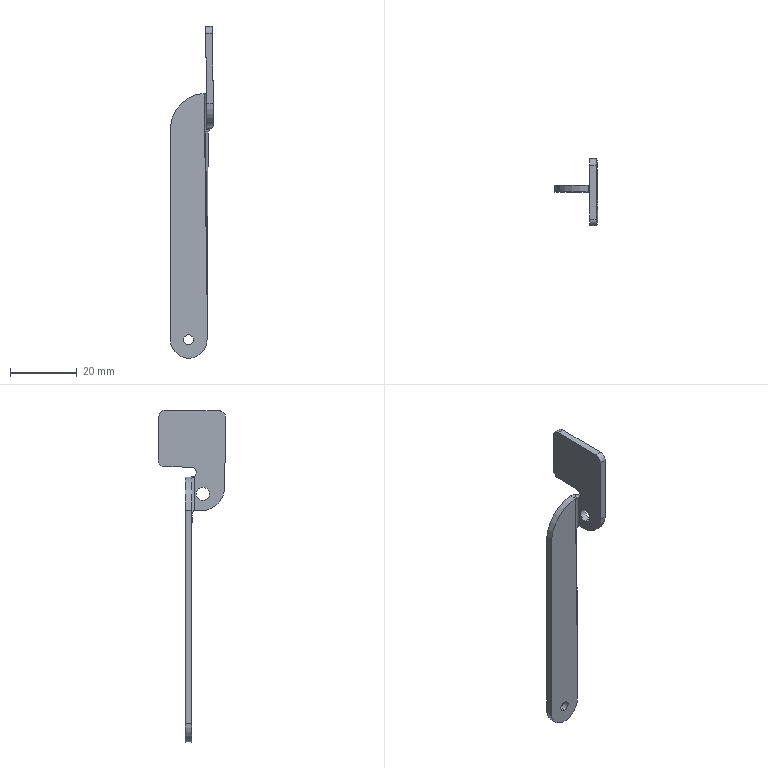Part | SolidWorks | features Fillet 5, HoleWzd 2, BaseBody 1, ICE 1 | 1 solid | 34 faces | box 13 x 20.187 x 99.625 mm | volume 2561 mm3 | cylinder 18 | plane 11 | spline 5 | commonest cylinder face diameters 4 x7 2 x2 3.001 x2 14 x2 1.473 x1 3.342 x1
STEP:
#1=CARTESIAN_POINT('',(79.957,-4.847,99.941));
#2=VERTEX_POINT('',#1);
#3=CARTESIAN_POINT('',(79.856,-11.846,106.839));
#4=VERTEX_POINT('',#3);
#5=CARTESIAN_POINT('',(79.855,-4.847,106.94));
#6=DIRECTION('',(-0.9999,0.,-0.01455));
#7=DIRECTION('',(0.01455,0.,-0.9999));
#8=AXIS2_PLACEMENT_3D('',#5,#6,#7);
#9=CIRCLE('',#8,7.);
#10=EDGE_CURVE('',#2,#4,#9,.T.);
#11=ORIENTED_EDGE('',*,*,#10,.F.);
#12=CARTESIAN_POINT('',(81.956,-4.847,99.97));
#13=VERTEX_POINT('',#12);
#14=CARTESIAN_POINT('',(79.957,-4.847,99.941));
#15=DIRECTION('',(0.9999,0.,0.01455));
#16=VECTOR('',#15,1000.);
#17=LINE('',#14,#16);
#18=EDGE_CURVE('',#2,#13,#17,.T.);
#19=ORIENTED_EDGE('',*,*,#18,.T.);
#20=CARTESIAN_POINT('',(81.856,-11.846,106.868));
#21=VERTEX_POINT('',#20);
#22=CARTESIAN_POINT('',(81.855,-4.847,106.969));
#23=DIRECTION('',(0.9999,0.,0.01455));
#24=DIRECTION('',(0.01455,0.,-0.9999));
#25=AXIS2_PLACEMENT_3D('',#22,#23,#24);
#26=CIRCLE('',#25,7.);
#27=EDGE_CURVE('',#21,#13,#26,.T.);
#28=ORIENTED_EDGE('',*,*,#27,.F.);
#29=CARTESIAN_POINT('',(79.856,-11.846,106.839));
#30=DIRECTION('',(0.9999,0.,0.01455));
#31=VECTOR('',#30,1000.);
#32=LINE('',#29,#31);
#33=EDGE_CURVE('',#4,#21,#32,.T.);
#34=ORIENTED_EDGE('',*,*,#33,.F.);
#35=EDGE_LOOP('',(#11,#19,#28,#34));
#36=FACE_OUTER_BOUND('',#35,.T.);
#37=CARTESIAN_POINT('',(79.855,-4.847,106.94));
#38=DIRECTION('',(0.9999,0.,0.01455));
#39=DIRECTION('',(0.01455,0.,-0.9999));
#40=AXIS2_PLACEMENT_3D('',#37,#38,#39);
#41=CYLINDRICAL_SURFACE('',#40,7.);
#42=ADVANCED_FACE('',(#36),#41,.T.);
#43=CARTESIAN_POINT('',(81.518,5.846,130.125));
#44=VERTEX_POINT('',#43);
#45=CARTESIAN_POINT('',(81.518,5.817,130.125));
#46=VERTEX_POINT('',#45);
#47=CARTESIAN_POINT('',(81.547,5.846,128.125));
#48=DIRECTION('',(0.9999,0.,0.01455));
#49=DIRECTION('',(0.01455,0.,-0.9999));
#50=AXIS2_PLACEMENT_3D('',#47,#48,#49);
#51=CIRCLE('',#50,2.);
#52=EDGE_CURVE('',#44,#46,#51,.T.);
#53=ORIENTED_EDGE('',*,*,#52,.F.);
#54=CARTESIAN_POINT('',(79.518,5.846,130.096));
#55=VERTEX_POINT('',#54);
#56=CARTESIAN_POINT('',(-1.875,5.846,128.912));
#57=DIRECTION('',(-0.9999,0.,-0.01455));
#58=VECTOR('',#57,1000.);
#59=LINE('',#56,#58);
#60=EDGE_CURVE('',#44,#55,#59,.T.);
#61=ORIENTED_EDGE('',*,*,#60,.T.);
#62=CARTESIAN_POINT('',(79.518,5.817,130.095));
#63=VERTEX_POINT('',#62);
#64=CARTESIAN_POINT('',(79.547,5.846,128.096));
#65=DIRECTION('',(-0.9999,0.,-0.01455));
#66=DIRECTION('',(0.01455,0.,-0.9999));
#67=AXIS2_PLACEMENT_3D('',#64,#65,#66);
#68=CIRCLE('',#67,2.);
#69=EDGE_CURVE('',#63,#55,#68,.T.);
#70=ORIENTED_EDGE('',*,*,#69,.F.);
#71=CARTESIAN_POINT('',(79.518,5.817,130.095));
#72=DIRECTION('',(-0.9999,0.,-0.01455));
#73=VECTOR('',#72,1000.);
#74=LINE('',#71,#73);
#75=EDGE_CURVE('',#46,#63,#74,.T.);
#76=ORIENTED_EDGE('',*,*,#75,.F.);
#77=EDGE_LOOP('',(#53,#61,#70,#76));
#78=FACE_OUTER_BOUND('',#77,.T.);
#79=CARTESIAN_POINT('',(-1.846,5.846,126.912));
#80=DIRECTION('',(-0.9999,0.,-0.01455));
#81=DIRECTION('',(-0.01455,0.,0.9999));
#82=AXIS2_PLACEMENT_3D('',#79,#80,#81);
#83=CYLINDRICAL_SURFACE('',#82,2.);
#84=ADVANCED_FACE('',(#78),#83,.T.);
#85=CARTESIAN_POINT('',(79.855,-5.318,106.933));
#86=VERTEX_POINT('',#85);
#87=CARTESIAN_POINT('',(79.913,-5.318,102.934));
#88=VERTEX_POINT('',#87);
#89=CARTESIAN_POINT('',(79.884,-5.318,104.933));
#90=DIRECTION('',(0.9999,0.,0.01455));
#91=DIRECTION('',(0.01455,0.,-0.9999));
#92=AXIS2_PLACEMENT_3D('',#89,#90,#91);
#93=CIRCLE('',#92,2.);
#94=EDGE_CURVE('',#86,#88,#93,.T.);
#95=ORIENTED_EDGE('',*,*,#94,.F.);
#96=CARTESIAN_POINT('',(81.855,-5.318,106.962));
#97=VERTEX_POINT('',#96);
#98=CARTESIAN_POINT('',(81.855,-5.318,106.962));
#99=DIRECTION('',(0.9999,0.,0.01455));
#100=VECTOR('',#99,1000.);
#101=LINE('',#98,#100);
#102=EDGE_CURVE('',#86,#97,#101,.T.);
#103=ORIENTED_EDGE('',*,*,#102,.T.);
#104=CARTESIAN_POINT('',(81.913,-5.318,102.963));
#105=VERTEX_POINT('',#104);
#106=CARTESIAN_POINT('',(81.884,-5.318,104.963));
#107=DIRECTION('',(0.9999,0.,0.01455));
#108=DIRECTION('',(0.01455,0.,-0.9999));
#109=AXIS2_PLACEMENT_3D('',#106,#107,#108);
#110=CIRCLE('',#109,2.);
#111=EDGE_CURVE('',#97,#105,#110,.T.);
#112=ORIENTED_EDGE('',*,*,#111,.T.);
#113=CARTESIAN_POINT('',(81.913,-5.318,102.963));
#114=DIRECTION('',(0.9999,0.,0.01455));
#115=VECTOR('',#114,1000.);
#116=LINE('',#113,#115);
#117=EDGE_CURVE('',#88,#105,#116,.T.);
#118=ORIENTED_EDGE('',*,*,#117,.F.);
#119=EDGE_LOOP('',(#95,#103,#112,#118));
#120=FACE_OUTER_BOUND('',#119,.T.);
#121=CARTESIAN_POINT('',(81.884,-5.318,104.963));
#122=DIRECTION('',(0.9999,0.,0.01455));
#123=DIRECTION('',(0.01455,0.,-0.9999));
#124=AXIS2_PLACEMENT_3D('',#121,#122,#123);
#125=CYLINDRICAL_SURFACE('',#124,2.);
#126=ADVANCED_FACE('',(#120),#125,.F.);
#127=CARTESIAN_POINT('',(74.456,-2.,34.499));
#128=VERTEX_POINT('',#127);
#129=CARTESIAN_POINT('',(74.456,-2.,37.501));
#130=VERTEX_POINT('',#129);
#131=CARTESIAN_POINT('',(74.456,-2.,36.));
#132=DIRECTION('',(0.,1.,0.));
#133=DIRECTION('',(0.,0.,1.));
#134=AXIS2_PLACEMENT_3D('',#131,#132,#133);
#135=CIRCLE('',#134,1.501);
#136=EDGE_CURVE('',#128,#130,#135,.T.);
#137=ORIENTED_EDGE('',*,*,#136,.F.);
#138=CARTESIAN_POINT('',(74.456,0.,34.499));
#139=VERTEX_POINT('',#138);
#140=CARTESIAN_POINT('',(74.456,0.,34.499));
#141=DIRECTION('',(0.,1.,0.));
#142=VECTOR('',#141,1000.);
#143=LINE('',#140,#142);
#144=EDGE_CURVE('',#128,#139,#143,.T.);
#145=ORIENTED_EDGE('',*,*,#144,.T.);
#146=CARTESIAN_POINT('',(74.456,0.,37.501));
#147=VERTEX_POINT('',#146);
#148=CARTESIAN_POINT('',(74.456,0.,36.));
#149=DIRECTION('',(0.,1.,0.));
#150=DIRECTION('',(0.,0.,1.));
#151=AXIS2_PLACEMENT_3D('',#148,#149,#150);
#152=CIRCLE('',#151,1.501);
#153=EDGE_CURVE('',#139,#147,#152,.T.);
#154=ORIENTED_EDGE('',*,*,#153,.T.);
#155=CARTESIAN_POINT('',(74.456,0.,37.501));
#156=DIRECTION('',(0.,1.,0.));
#157=VECTOR('',#156,1000.);
#158=LINE('',#155,#157);
#159=EDGE_CURVE('',#130,#147,#158,.T.);
#160=ORIENTED_EDGE('',*,*,#159,.F.);
#161=EDGE_LOOP('',(#137,#145,#154,#160));
#162=FACE_OUTER_BOUND('',#161,.T.);
#163=CARTESIAN_POINT('',(74.456,0.,36.));
#164=DIRECTION('',(0.,1.,0.));
#165=DIRECTION('',(0.,0.,1.));
#166=AXIS2_PLACEMENT_3D('',#163,#164,#165);
#167=CYLINDRICAL_SURFACE('',#166,1.501);
#168=ADVANCED_FACE('',(#162),#167,.F.);
#169=CARTESIAN_POINT('',(79.884,-5.318,104.933));
#170=DIRECTION('',(0.9999,0.,0.01455));
#171=DIRECTION('',(0.01455,0.,-0.9999));
#172=AXIS2_PLACEMENT_3D('',#169,#170,#171);
#173=CIRCLE('',#172,2.);
#174=EDGE_CURVE('',#88,#86,#173,.T.);
#175=ORIENTED_EDGE('',*,*,#174,.T.);
#176=ORIENTED_EDGE('',*,*,#94,.T.);
#177=EDGE_LOOP('',(#175,#176));
#178=FACE_BOUND('',#177,.T.);
#179=CARTESIAN_POINT('',(79.957,-4.745,99.942));
#180=VERTEX_POINT('',#179);
#181=CARTESIAN_POINT('',(79.956,-2.745,99.971));
#182=VERTEX_POINT('',#181);
#183=CARTESIAN_POINT('',(79.956,-2.745,99.971));
#184=DIRECTION('',(-0.0002116,0.9999,0.01455));
#185=VECTOR('',#184,1000.);
#186=LINE('',#183,#185);
#187=EDGE_CURVE('',#180,#182,#186,.T.);
#188=ORIENTED_EDGE('',*,*,#187,.F.);
#189=CARTESIAN_POINT('',(79.855,-4.847,106.94));
#190=DIRECTION('',(-0.9999,0.,-0.01455));
#191=DIRECTION('',(0.01455,0.,-0.9999));
#192=AXIS2_PLACEMENT_3D('',#189,#190,#191);
#193=CIRCLE('',#192,7.);
#194=EDGE_CURVE('',#180,#2,#193,.T.);
#195=ORIENTED_EDGE('',*,*,#194,.T.);
#196=ORIENTED_EDGE('',*,*,#10,.T.);
#197=CARTESIAN_POINT('',(79.551,-12.152,127.834));
#198=VERTEX_POINT('',#197);
#199=CARTESIAN_POINT('',(79.856,-11.846,106.839));
#200=DIRECTION('',(0.01455,0.01455,-0.9998));
#201=VECTOR('',#200,1000.);
#202=LINE('',#199,#201);
#203=EDGE_CURVE('',#198,#4,#202,.T.);
#204=ORIENTED_EDGE('',*,*,#203,.F.);
#205=CARTESIAN_POINT('',(79.521,-10.181,129.863));
#206=VERTEX_POINT('',#205);
#207=CARTESIAN_POINT('',(79.55,-10.152,127.863));
#208=DIRECTION('',(-0.9999,0.,-0.01455));
#209=DIRECTION('',(0.01455,0.,-0.9999));
#210=AXIS2_PLACEMENT_3D('',#207,#208,#209);
#211=CIRCLE('',#210,2.);
#212=EDGE_CURVE('',#198,#206,#211,.T.);
#213=ORIENTED_EDGE('',*,*,#212,.T.);
#214=CARTESIAN_POINT('',(79.521,-10.181,129.863));
#215=DIRECTION('',(0.0002116,-0.9999,-0.01455));
#216=VECTOR('',#215,1000.);
#217=LINE('',#214,#216);
#218=EDGE_CURVE('',#63,#206,#217,.T.);
#219=ORIENTED_EDGE('',*,*,#218,.F.);
#220=ORIENTED_EDGE('',*,*,#69,.T.);
#221=CARTESIAN_POINT('',(79.547,7.846,128.125));
#222=VERTEX_POINT('',#221);
#223=CARTESIAN_POINT('',(79.547,5.846,128.096));
#224=DIRECTION('',(-0.9999,0.,-0.01455));
#225=DIRECTION('',(0.01455,0.,-0.9999));
#226=AXIS2_PLACEMENT_3D('',#223,#224,#225);
#227=CIRCLE('',#226,2.);
#228=EDGE_CURVE('',#55,#222,#227,.T.);
#229=ORIENTED_EDGE('',*,*,#228,.T.);
#230=CARTESIAN_POINT('',(79.736,8.035,115.128));
#231=VERTEX_POINT('',#230);
#232=CARTESIAN_POINT('',(79.517,7.817,130.125));
#233=DIRECTION('',(-0.01455,-0.01455,0.9998));
#234=VECTOR('',#233,1000.);
#235=LINE('',#232,#234);
#236=EDGE_CURVE('',#231,#222,#235,.T.);
#237=ORIENTED_EDGE('',*,*,#236,.F.);
#238=CARTESIAN_POINT('',(79.765,6.065,113.099));
#239=VERTEX_POINT('',#238);
#240=CARTESIAN_POINT('',(79.736,6.035,115.099));
#241=DIRECTION('',(-0.9999,0.,-0.01455));
#242=DIRECTION('',(0.01455,0.,-0.9999));
#243=AXIS2_PLACEMENT_3D('',#240,#241,#242);
#244=CIRCLE('',#243,2.);
#245=EDGE_CURVE('',#231,#239,#244,.T.);
#246=ORIENTED_EDGE('',*,*,#245,.T.);
#247=CARTESIAN_POINT('',(79.767,-2.118,112.98));
#248=VERTEX_POINT('',#247);
#249=CARTESIAN_POINT('',(79.765,8.064,113.128));
#250=DIRECTION('',(0.0002116,-0.9999,-0.01455));
#251=VECTOR('',#250,1000.);
#252=LINE('',#249,#251);
#253=EDGE_CURVE('',#239,#248,#252,.T.);
#254=ORIENTED_EDGE('',*,*,#253,.T.);
#255=CARTESIAN_POINT('',(79.771,-2.782,112.716));
#256=VERTEX_POINT('',#255);
#257=CARTESIAN_POINT('',(79.781,-2.104,111.98));
#258=DIRECTION('',(0.9999,0.,0.01455));
#259=DIRECTION('',(0.01455,0.,-0.9999));
#260=AXIS2_PLACEMENT_3D('',#257,#258,#259);
#261=CIRCLE('',#260,1.);
#262=EDGE_CURVE('',#248,#256,#261,.T.);
#263=ORIENTED_EDGE('',*,*,#262,.T.);
#264=CARTESIAN_POINT('',(79.807,-2.745,110.226));
#265=VERTEX_POINT('',#264);
#266=CARTESIAN_POINT('',(79.789,-1.649,111.487));
#267=DIRECTION('',(-0.9999,0.,-0.01455));
#268=DIRECTION('',(-0.01455,-0.01455,0.9998));
#269=AXIS2_PLACEMENT_3D('',#266,#267,#268);
#270=CIRCLE('',#269,1.671);
#271=EDGE_CURVE('',#265,#256,#270,.T.);
#272=ORIENTED_EDGE('',*,*,#271,.F.);
#273=CARTESIAN_POINT('',(79.807,-2.737,110.218));
#274=VERTEX_POINT('',#273);
#275=CARTESIAN_POINT('',(79.796,-2.089,110.98));
#276=DIRECTION('',(-0.9999,0.,-0.01455));
#277=DIRECTION('',(-0.01455,-0.01455,0.9998));
#278=AXIS2_PLACEMENT_3D('',#275,#276,#277);
#279=CIRCLE('',#278,1.);
#280=EDGE_CURVE('',#274,#265,#279,.T.);
#281=ORIENTED_EDGE('',*,*,#280,.F.);
#282=CARTESIAN_POINT('',(79.956,-2.737,99.971));
#283=VERTEX_POINT('',#282);
#284=CARTESIAN_POINT('',(79.965,-2.737,99.398));
#285=DIRECTION('',(0.01455,0.,-0.9999));
#286=VECTOR('',#285,1000.);
#287=LINE('',#284,#286);
#288=EDGE_CURVE('',#274,#283,#287,.T.);
#289=ORIENTED_EDGE('',*,*,#288,.T.);
#290=CARTESIAN_POINT('',(79.985,-2.716,97.971));
#291=DIRECTION('',(-0.9999,0.,-0.01455));
#292=DIRECTION('',(-0.01455,-0.01455,0.9998));
#293=AXIS2_PLACEMENT_3D('',#290,#291,#292);
#294=CIRCLE('',#293,2.);
#295=EDGE_CURVE('',#182,#283,#294,.T.);
#296=ORIENTED_EDGE('',*,*,#295,.F.);
#297=EDGE_LOOP('',(#188,#195,#196,#204,#213,#219,#220,#229,#237,#246,#254,#263,#272,#281,#289,#296));
#298=FACE_OUTER_BOUND('',#297,.T.);
#299=CARTESIAN_POINT('',(79.796,-2.089,110.98));
#300=DIRECTION('',(0.9999,0.,0.01455));
#301=DIRECTION('',(-0.01455,-0.01455,0.9998));
#302=AXIS2_PLACEMENT_3D('',#299,#300,#301);
#303=PLANE('',#302);
#304=ADVANCED_FACE('',(#178,#298),#303,.F.);
#305=CARTESIAN_POINT('',(81.521,-10.181,129.892));
#306=VERTEX_POINT('',#305);
#307=CARTESIAN_POINT('',(81.521,-10.181,129.892));
#308=DIRECTION('',(0.0002116,-0.9999,-0.01455));
#309=VECTOR('',#308,1000.);
#310=LINE('',#307,#309);
#311=EDGE_CURVE('',#46,#306,#310,.T.);
#312=ORIENTED_EDGE('',*,*,#311,.F.);
#313=ORIENTED_EDGE('',*,*,#75,.T.);
#314=ORIENTED_EDGE('',*,*,#218,.T.);
#315=CARTESIAN_POINT('',(79.521,-10.181,129.863));
#316=DIRECTION('',(0.9999,0.,0.01455));
#317=VECTOR('',#316,1000.);
#318=LINE('',#315,#317);
#319=EDGE_CURVE('',#206,#306,#318,.T.);
#320=ORIENTED_EDGE('',*,*,#319,.T.);
#321=EDGE_LOOP('',(#312,#313,#314,#320));
#322=FACE_OUTER_BOUND('',#321,.T.);
#323=CARTESIAN_POINT('',(79.521,-10.181,129.863));
#324=DIRECTION('',(-0.01455,-0.01455,0.9998));
#325=DIRECTION('',(0.0002116,-0.9999,-0.01455));
#326=AXIS2_PLACEMENT_3D('',#323,#324,#325);
#327=PLANE('',#326);
#328=ADVANCED_FACE('',(#322),#327,.T.);
#329=CARTESIAN_POINT('',(81.884,-5.318,104.963));
#330=DIRECTION('',(0.9999,0.,0.01455));
#331=DIRECTION('',(0.01455,0.,-0.9999));
#332=AXIS2_PLACEMENT_3D('',#329,#330,#331);
#333=CIRCLE('',#332,2.);
#334=EDGE_CURVE('',#105,#97,#333,.T.);
#335=ORIENTED_EDGE('',*,*,#334,.F.);
#336=ORIENTED_EDGE('',*,*,#111,.F.);
#337=EDGE_LOOP('',(#335,#336));
#338=FACE_BOUND('',#337,.T.);
#339=CARTESIAN_POINT('',(81.551,-12.152,127.863));
#340=VERTEX_POINT('',#339);
#341=CARTESIAN_POINT('',(81.856,-11.846,106.868));
#342=DIRECTION('',(0.01455,0.01455,-0.9998));
#343=VECTOR('',#342,1000.);
#344=LINE('',#341,#343);
#345=EDGE_CURVE('',#340,#21,#344,.T.);
#346=ORIENTED_EDGE('',*,*,#345,.T.);
#347=ORIENTED_EDGE('',*,*,#27,.T.);
#348=CARTESIAN_POINT('',(81.956,-4.745,99.971));
#349=VERTEX_POINT('',#348);
#350=CARTESIAN_POINT('',(81.855,-4.847,106.969));
#351=DIRECTION('',(0.9999,0.,0.01455));
#352=DIRECTION('',(0.01455,0.,-0.9999));
#353=AXIS2_PLACEMENT_3D('',#350,#351,#352);
#354=CIRCLE('',#353,7.);
#355=EDGE_CURVE('',#13,#349,#354,.T.);
#356=ORIENTED_EDGE('',*,*,#355,.T.);
#357=CARTESIAN_POINT('',(81.956,-2.745,100.));
#358=VERTEX_POINT('',#357);
#359=CARTESIAN_POINT('',(81.956,-2.745,100.));
#360=DIRECTION('',(-0.0002116,0.9999,0.01455));
#361=VECTOR('',#360,1000.);
#362=LINE('',#359,#361);
#363=EDGE_CURVE('',#349,#358,#362,.T.);
#364=ORIENTED_EDGE('',*,*,#363,.T.);
#365=CARTESIAN_POINT('',(81.956,-2.737,100.));
#366=VERTEX_POINT('',#365);
#367=CARTESIAN_POINT('',(81.985,-2.716,98.));
#368=DIRECTION('',(-0.9999,0.,-0.01455));
#369=DIRECTION('',(-0.01455,-0.01455,0.9998));
#370=AXIS2_PLACEMENT_3D('',#367,#368,#369);
#371=CIRCLE('',#370,2.);
#372=EDGE_CURVE('',#358,#366,#371,.T.);
#373=ORIENTED_EDGE('',*,*,#372,.T.);
#374=CARTESIAN_POINT('',(81.807,-2.737,110.247));
#375=VERTEX_POINT('',#374);
#376=CARTESIAN_POINT('',(81.796,-2.737,111.01));
#377=DIRECTION('',(-0.01455,0.,0.9999));
#378=VECTOR('',#377,1000.);
#379=LINE('',#376,#378);
#380=EDGE_CURVE('',#366,#375,#379,.T.);
#381=ORIENTED_EDGE('',*,*,#380,.T.);
#382=CARTESIAN_POINT('',(81.807,-2.745,110.255));
#383=VERTEX_POINT('',#382);
#384=CARTESIAN_POINT('',(81.796,-2.089,111.01));
#385=DIRECTION('',(-0.9999,0.,-0.01455));
#386=DIRECTION('',(-0.01455,-0.01455,0.9998));
#387=AXIS2_PLACEMENT_3D('',#384,#385,#386);
#388=CIRCLE('',#387,1.);
#389=EDGE_CURVE('',#375,#383,#388,.T.);
#390=ORIENTED_EDGE('',*,*,#389,.T.);
#391=CARTESIAN_POINT('',(81.771,-2.782,112.745));
#392=VERTEX_POINT('',#391);
#393=CARTESIAN_POINT('',(81.788,-1.649,111.516));
#394=DIRECTION('',(-0.9999,0.,-0.01455));
#395=DIRECTION('',(-0.01455,-0.01455,0.9998));
#396=AXIS2_PLACEMENT_3D('',#393,#394,#395);
#397=CIRCLE('',#396,1.671);
#398=EDGE_CURVE('',#383,#392,#397,.T.);
#399=ORIENTED_EDGE('',*,*,#398,.T.);
#400=CARTESIAN_POINT('',(81.767,-2.118,113.009));
#401=VERTEX_POINT('',#400);
#402=CARTESIAN_POINT('',(81.781,-2.104,112.009));
#403=DIRECTION('',(-0.9999,0.,-0.01455));
#404=DIRECTION('',(0.01455,0.,-0.9999));
#405=AXIS2_PLACEMENT_3D('',#402,#403,#404);
#406=CIRCLE('',#405,1.);
#407=EDGE_CURVE('',#392,#401,#406,.T.);
#408=ORIENTED_EDGE('',*,*,#407,.T.);
#409=CARTESIAN_POINT('',(81.765,6.065,113.128));
#410=VERTEX_POINT('',#409);
#411=CARTESIAN_POINT('',(81.765,8.064,113.157));
#412=DIRECTION('',(0.0002116,-0.9999,-0.01455));
#413=VECTOR('',#412,1000.);
#414=LINE('',#411,#413);
#415=EDGE_CURVE('',#410,#401,#414,.T.);
#416=ORIENTED_EDGE('',*,*,#415,.F.);
#417=CARTESIAN_POINT('',(81.735,8.035,115.157));
#418=VERTEX_POINT('',#417);
#419=CARTESIAN_POINT('',(81.736,6.035,115.128));
#420=DIRECTION('',(0.9999,0.,0.01455));
#421=DIRECTION('',(0.01455,0.,-0.9999));
#422=AXIS2_PLACEMENT_3D('',#419,#420,#421);
#423=CIRCLE('',#422,2.);
#424=EDGE_CURVE('',#410,#418,#423,.T.);
#425=ORIENTED_EDGE('',*,*,#424,.T.);
#426=CARTESIAN_POINT('',(81.546,7.846,128.154));
#427=VERTEX_POINT('',#426);
#428=CARTESIAN_POINT('',(81.765,8.064,113.157));
#429=DIRECTION('',(0.01455,0.01455,-0.9998));
#430=VECTOR('',#429,1000.);
#431=LINE('',#428,#430);
#432=EDGE_CURVE('',#427,#418,#431,.T.);
#433=ORIENTED_EDGE('',*,*,#432,.F.);
#434=CARTESIAN_POINT('',(81.547,5.846,128.125));
#435=DIRECTION('',(0.9999,0.,0.01455));
#436=DIRECTION('',(0.01455,0.,-0.9999));
#437=AXIS2_PLACEMENT_3D('',#434,#435,#436);
#438=CIRCLE('',#437,2.);
#439=EDGE_CURVE('',#427,#44,#438,.T.);
#440=ORIENTED_EDGE('',*,*,#439,.T.);
#441=ORIENTED_EDGE('',*,*,#52,.T.);
#442=ORIENTED_EDGE('',*,*,#311,.T.);
#443=CARTESIAN_POINT('',(81.55,-10.152,127.892));
#444=DIRECTION('',(0.9999,0.,0.01455));
#445=DIRECTION('',(0.01455,0.,-0.9999));
#446=AXIS2_PLACEMENT_3D('',#443,#444,#445);
#447=CIRCLE('',#446,2.);
#448=EDGE_CURVE('',#306,#340,#447,.T.);
#449=ORIENTED_EDGE('',*,*,#448,.T.);
#450=EDGE_LOOP('',(#346,#347,#356,#364,#373,#381,#390,#399,#408,#416,#425,#433,#440,#441,#442,#449));
#451=FACE_OUTER_BOUND('',#450,.T.);
#452=CARTESIAN_POINT('',(81.796,-2.089,111.01));
#453=DIRECTION('',(0.9999,0.,0.01455));
#454=DIRECTION('',(-0.01455,-0.01455,0.9998));
#455=AXIS2_PLACEMENT_3D('',#452,#453,#454);
#456=PLANE('',#455);
#457=ADVANCED_FACE('',(#338,#451),#456,.T.);
#458=CARTESIAN_POINT('',(79.807,-2.737,110.218));
#459=CARTESIAN_POINT('',(81.807,-2.737,110.247));
#460=B_SPLINE_CURVE_WITH_KNOTS('',1,(#458,#459),.UNSPECIFIED.,.F.,.F.,(2,2),(0.,1.),.UNSPECIFIED.);
#461=EDGE_CURVE('',#274,#375,#460,.T.);
#462=ORIENTED_EDGE('',*,*,#461,.F.);
#463=ORIENTED_EDGE('',*,*,#280,.T.);
#464=CARTESIAN_POINT('',(79.807,-2.745,110.226));
#465=DIRECTION('',(0.9999,0.,0.01455));
#466=VECTOR('',#465,1000.);
#467=LINE('',#464,#466);
#468=EDGE_CURVE('',#265,#383,#467,.T.);
#469=ORIENTED_EDGE('',*,*,#468,.T.);
#470=ORIENTED_EDGE('',*,*,#389,.F.);
#471=EDGE_LOOP('',(#462,#463,#469,#470));
#472=FACE_OUTER_BOUND('',#471,.T.);
#473=CARTESIAN_POINT('',(79.796,-2.089,110.98));
#474=DIRECTION('',(0.9999,0.,0.01455));
#475=DIRECTION('',(-0.01455,-0.01455,0.9998));
#476=AXIS2_PLACEMENT_3D('',#473,#474,#475);
#477=CYLINDRICAL_SURFACE('',#476,1.);
#478=ADVANCED_FACE('',(#472),#477,.F.);
#479=CARTESIAN_POINT('',(81.956,-2.737,100.));
#480=CARTESIAN_POINT('',(79.956,-2.737,99.971));
#481=B_SPLINE_CURVE_WITH_KNOTS('',1,(#479,#480),.UNSPECIFIED.,.F.,.F.,(2,2),(0.,1.),.UNSPECIFIED.);
#482=EDGE_CURVE('',#366,#283,#481,.T.);
#483=ORIENTED_EDGE('',*,*,#482,.F.);
#484=ORIENTED_EDGE('',*,*,#372,.F.);
#485=CARTESIAN_POINT('',(79.956,-2.745,99.971));
#486=DIRECTION('',(0.9999,0.,0.01455));
#487=VECTOR('',#486,1000.);
#488=LINE('',#485,#487);
#489=EDGE_CURVE('',#182,#358,#488,.T.);
#490=ORIENTED_EDGE('',*,*,#489,.F.);
#491=ORIENTED_EDGE('',*,*,#295,.T.);
#492=EDGE_LOOP('',(#483,#484,#490,#491));
#493=FACE_OUTER_BOUND('',#492,.T.);
#494=CARTESIAN_POINT('',(79.985,-2.716,97.971));
#495=DIRECTION('',(0.9999,0.,0.01455));
#496=DIRECTION('',(-0.01455,-0.01455,0.9998));
#497=AXIS2_PLACEMENT_3D('',#494,#495,#496);
#498=CYLINDRICAL_SURFACE('',#497,2.);
#499=ADVANCED_FACE('',(#493),#498,.F.);
#500=ORIENTED_EDGE('',*,*,#363,.F.);
#501=CARTESIAN_POINT('',(79.957,-4.745,99.942));
#502=DIRECTION('',(-0.9999,0.,-0.01455));
#503=VECTOR('',#502,1000.);
#504=LINE('',#501,#503);
#505=EDGE_CURVE('',#349,#180,#504,.T.);
#506=ORIENTED_EDGE('',*,*,#505,.T.);
#507=ORIENTED_EDGE('',*,*,#187,.T.);
#508=ORIENTED_EDGE('',*,*,#489,.T.);
#509=EDGE_LOOP('',(#500,#506,#507,#508));
#510=FACE_OUTER_BOUND('',#509,.T.);
#511=CARTESIAN_POINT('',(79.956,-2.745,99.971));
#512=DIRECTION('',(0.01455,0.01455,-0.9998));
#513=DIRECTION('',(-0.0002116,0.9999,0.01455));
#514=AXIS2_PLACEMENT_3D('',#511,#512,#513);
#515=PLANE('',#514);
#516=ADVANCED_FACE('',(#510),#515,.T.);
#517=ORIENTED_EDGE('',*,*,#203,.T.);
#518=ORIENTED_EDGE('',*,*,#33,.T.);
#519=ORIENTED_EDGE('',*,*,#345,.F.);
#520=CARTESIAN_POINT('',(79.551,-12.152,127.834));
#521=DIRECTION('',(-0.9999,0.,-0.01455));
#522=VECTOR('',#521,1000.);
#523=LINE('',#520,#522);
#524=EDGE_CURVE('',#340,#198,#523,.T.);
#525=ORIENTED_EDGE('',*,*,#524,.T.);
#526=EDGE_LOOP('',(#517,#518,#519,#525));
#527=FACE_OUTER_BOUND('',#526,.T.);
#528=CARTESIAN_POINT('',(79.856,-11.846,106.839));
#529=DIRECTION('',(0.0002116,-0.9999,-0.01455));
#530=DIRECTION('',(0.01455,0.01455,-0.9998));
#531=AXIS2_PLACEMENT_3D('',#528,#529,#530);
#532=PLANE('',#531);
#533=ADVANCED_FACE('',(#527),#532,.T.);
#534=ORIENTED_EDGE('',*,*,#271,.T.);
#535=CARTESIAN_POINT('',(79.771,-2.782,112.716));
#536=DIRECTION('',(0.9999,0.,0.01455));
#537=VECTOR('',#536,1000.);
#538=LINE('',#535,#537);
#539=EDGE_CURVE('',#256,#392,#538,.T.);
#540=ORIENTED_EDGE('',*,*,#539,.T.);
#541=ORIENTED_EDGE('',*,*,#398,.F.);
#542=ORIENTED_EDGE('',*,*,#468,.F.);
#543=EDGE_LOOP('',(#534,#540,#541,#542));
#544=FACE_OUTER_BOUND('',#543,.T.);
#545=CARTESIAN_POINT('',(79.789,-1.649,111.487));
#546=DIRECTION('',(0.9999,0.,0.01455));
#547=DIRECTION('',(-0.01455,-0.01455,0.9998));
#548=AXIS2_PLACEMENT_3D('',#545,#546,#547);
#549=CYLINDRICAL_SURFACE('',#548,1.671);
#550=ADVANCED_FACE('',(#544),#549,.F.);
#551=CARTESIAN_POINT('',(79.956,0.,36.));
#552=VERTEX_POINT('',#551);
#553=CARTESIAN_POINT('',(68.956,0.,36.));
#554=VERTEX_POINT('',#553);
#555=CARTESIAN_POINT('',(74.456,0.,36.));
#556=DIRECTION('',(0.,1.,0.));
#557=DIRECTION('',(0.,0.,-1.));
#558=AXIS2_PLACEMENT_3D('',#555,#556,#557);
#559=CIRCLE('',#558,5.5);
#560=EDGE_CURVE('',#552,#554,#559,.T.);
#561=ORIENTED_EDGE('',*,*,#560,.F.);
#562=CARTESIAN_POINT('',(79.956,-2.,36.));
#563=VERTEX_POINT('',#562);
#564=CARTESIAN_POINT('',(79.956,-2.,36.));
#565=DIRECTION('',(0.,1.,0.));
#566=VECTOR('',#565,1000.);
#567=LINE('',#564,#566);
#568=EDGE_CURVE('',#563,#552,#567,.T.);
#569=ORIENTED_EDGE('',*,*,#568,.F.);
#570=CARTESIAN_POINT('',(68.956,-2.,36.));
#571=VERTEX_POINT('',#570);
#572=CARTESIAN_POINT('',(74.456,-2.,36.));
#573=DIRECTION('',(0.,1.,0.));
#574=DIRECTION('',(0.,0.,-1.));
#575=AXIS2_PLACEMENT_3D('',#572,#573,#574);
#576=CIRCLE('',#575,5.5);
#577=EDGE_CURVE('',#563,#571,#576,.T.);
#578=ORIENTED_EDGE('',*,*,#577,.T.);
#579=CARTESIAN_POINT('',(68.956,-2.,36.));
#580=DIRECTION('',(0.,1.,0.));
#581=VECTOR('',#580,1000.);
#582=LINE('',#579,#581);
#583=EDGE_CURVE('',#571,#554,#582,.T.);
#584=ORIENTED_EDGE('',*,*,#583,.T.);
#585=EDGE_LOOP('',(#561,#569,#578,#584));
#586=FACE_OUTER_BOUND('',#585,.T.);
#587=CARTESIAN_POINT('',(74.456,-2.,36.));
#588=DIRECTION('',(0.,1.,0.));
#589=DIRECTION('',(0.,0.,1.));
#590=AXIS2_PLACEMENT_3D('',#587,#588,#589);
#591=CYLINDRICAL_SURFACE('',#590,5.5);
#592=ADVANCED_FACE('',(#586),#591,.T.);
#593=CARTESIAN_POINT('',(68.956,0.,100.));
#594=VERTEX_POINT('',#593);
#595=CARTESIAN_POINT('',(68.956,0.,100.));
#596=DIRECTION('',(0.,0.,1.));
#597=VECTOR('',#596,1000.);
#598=LINE('',#595,#597);
#599=EDGE_CURVE('',#554,#594,#598,.T.);
#600=ORIENTED_EDGE('',*,*,#599,.F.);
#601=ORIENTED_EDGE('',*,*,#583,.F.);
#602=CARTESIAN_POINT('',(68.956,-2.,100.));
#603=VERTEX_POINT('',#602);
#604=CARTESIAN_POINT('',(68.956,-2.,100.));
#605=DIRECTION('',(0.,0.,1.));
#606=VECTOR('',#605,1000.);
#607=LINE('',#604,#606);
#608=EDGE_CURVE('',#571,#603,#607,.T.);
#609=ORIENTED_EDGE('',*,*,#608,.T.);
#610=CARTESIAN_POINT('',(68.956,-2.,100.));
#611=DIRECTION('',(0.,1.,0.));
#612=VECTOR('',#611,1000.);
#613=LINE('',#610,#612);
#614=EDGE_CURVE('',#603,#594,#613,.T.);
#615=ORIENTED_EDGE('',*,*,#614,.T.);
#616=EDGE_LOOP('',(#600,#601,#609,#615));
#617=FACE_OUTER_BOUND('',#616,.T.);
#618=CARTESIAN_POINT('',(68.956,-2.,100.));
#619=DIRECTION('',(-1.,0.,0.));
#620=DIRECTION('',(0.,0.,1.));
#621=AXIS2_PLACEMENT_3D('',#618,#619,#620);
#622=PLANE('',#621);
#623=ADVANCED_FACE('',(#617),#622,.T.);
#624=CARTESIAN_POINT('',(74.456,-2.,36.));
#625=DIRECTION('',(0.,1.,0.));
#626=DIRECTION('',(0.,0.,1.));
#627=AXIS2_PLACEMENT_3D('',#624,#625,#626);
#628=CIRCLE('',#627,1.501);
#629=EDGE_CURVE('',#130,#128,#628,.T.);
#630=ORIENTED_EDGE('',*,*,#629,.T.);
#631=ORIENTED_EDGE('',*,*,#136,.T.);
#632=EDGE_LOOP('',(#630,#631));
#633=FACE_BOUND('',#632,.T.);
#634=CARTESIAN_POINT('',(79.956,-2.,49.349));
#635=VERTEX_POINT('',#634);
#636=CARTESIAN_POINT('',(79.956,-2.,98.));
#637=DIRECTION('',(0.,0.,-1.));
#638=VECTOR('',#637,1000.);
#639=LINE('',#636,#638);
#640=EDGE_CURVE('',#635,#563,#639,.T.);
#641=ORIENTED_EDGE('',*,*,#640,.F.);
#642=CARTESIAN_POINT('',(79.074,-2.,109.965));
#643=VERTEX_POINT('',#642);
#644=CARTESIAN_POINT('',(79.074,-2.,109.98));
#645=DIRECTION('',(-0.01455,0.,0.9999));
#646=VECTOR('',#645,1000.);
#647=LINE('',#644,#646);
#648=EDGE_CURVE('',#635,#643,#647,.T.);
#649=ORIENTED_EDGE('',*,*,#648,.T.);
#650=CARTESIAN_POINT('',(79.956,-2.,98.95));
#651=DIRECTION('',(0.,1.,0.));
#652=DIRECTION('',(0.,0.,-1.));
#653=AXIS2_PLACEMENT_3D('',#650,#651,#652);
#654=CIRCLE('',#653,11.05);
#655=EDGE_CURVE('',#603,#643,#654,.T.);
#656=ORIENTED_EDGE('',*,*,#655,.F.);
#657=ORIENTED_EDGE('',*,*,#608,.F.);
#658=ORIENTED_EDGE('',*,*,#577,.F.);
#659=EDGE_LOOP('',(#641,#649,#656,#657,#658));
#660=FACE_OUTER_BOUND('',#659,.T.);
#661=CARTESIAN_POINT('',(81.14,-2.,111.));
#662=DIRECTION('',(0.,1.,0.));
#663=DIRECTION('',(0.,0.,1.));
#664=AXIS2_PLACEMENT_3D('',#661,#662,#663);
#665=PLANE('',#664);
#666=ADVANCED_FACE('',(#633,#660),#665,.F.);
#667=ORIENTED_EDGE('',*,*,#655,.T.);
#668=CARTESIAN_POINT('',(79.074,0.,109.965));
#669=VERTEX_POINT('',#668);
#670=CARTESIAN_POINT('',(79.074,-2.,109.965));
#671=CARTESIAN_POINT('',(79.074,-1.333,109.965));
#672=CARTESIAN_POINT('',(79.074,-0.6667,109.965));
#673=CARTESIAN_POINT('',(79.074,0.,109.965));
#674=B_SPLINE_CURVE_WITH_KNOTS('',3,(#670,#671,#672,#673),.UNSPECIFIED.,.F.,.F.,(4,4),(0.,1.),.UNSPECIFIED.);
#675=EDGE_CURVE('',#643,#669,#674,.T.);
#676=ORIENTED_EDGE('',*,*,#675,.T.);
#677=CARTESIAN_POINT('',(79.956,0.,98.95));
#678=DIRECTION('',(0.,1.,0.));
#679=DIRECTION('',(0.,0.,-1.));
#680=AXIS2_PLACEMENT_3D('',#677,#678,#679);
#681=CIRCLE('',#680,11.05);
#682=EDGE_CURVE('',#594,#669,#681,.T.);
#683=ORIENTED_EDGE('',*,*,#682,.F.);
#684=ORIENTED_EDGE('',*,*,#614,.F.);
#685=EDGE_LOOP('',(#667,#676,#683,#684));
#686=FACE_OUTER_BOUND('',#685,.T.);
#687=CARTESIAN_POINT('',(79.956,-2.,98.95));
#688=DIRECTION('',(0.,1.,0.));
#689=DIRECTION('',(0.,0.,1.));
#690=AXIS2_PLACEMENT_3D('',#687,#688,#689);
#691=CYLINDRICAL_SURFACE('',#690,11.05);
#692=ADVANCED_FACE('',(#686),#691,.T.);
#693=CARTESIAN_POINT('',(74.456,0.,36.));
#694=DIRECTION('',(0.,1.,0.));
#695=DIRECTION('',(0.,0.,1.));
#696=AXIS2_PLACEMENT_3D('',#693,#694,#695);
#697=CIRCLE('',#696,1.501);
#698=EDGE_CURVE('',#147,#139,#697,.T.);
#699=ORIENTED_EDGE('',*,*,#698,.F.);
#700=ORIENTED_EDGE('',*,*,#153,.F.);
#701=EDGE_LOOP('',(#699,#700));
#702=FACE_BOUND('',#701,.T.);
#703=ORIENTED_EDGE('',*,*,#682,.T.);
#704=CARTESIAN_POINT('',(79.956,0.,49.349));
#705=VERTEX_POINT('',#704);
#706=CARTESIAN_POINT('',(79.059,0.,110.97));
#707=DIRECTION('',(0.01455,0.,-0.9999));
#708=VECTOR('',#707,1000.);
#709=LINE('',#706,#708);
#710=EDGE_CURVE('',#669,#705,#709,.T.);
#711=ORIENTED_EDGE('',*,*,#710,.T.);
#712=CARTESIAN_POINT('',(79.956,0.,98.));
#713=DIRECTION('',(0.,0.,-1.));
#714=VECTOR('',#713,1000.);
#715=LINE('',#712,#714);
#716=EDGE_CURVE('',#705,#552,#715,.T.);
#717=ORIENTED_EDGE('',*,*,#716,.T.);
#718=ORIENTED_EDGE('',*,*,#560,.T.);
#719=ORIENTED_EDGE('',*,*,#599,.T.);
#720=EDGE_LOOP('',(#703,#711,#717,#718,#719));
#721=FACE_OUTER_BOUND('',#720,.T.);
#722=CARTESIAN_POINT('',(81.14,0.,111.));
#723=DIRECTION('',(0.,1.,0.));
#724=DIRECTION('',(0.,0.,1.));
#725=AXIS2_PLACEMENT_3D('',#722,#723,#724);
#726=PLANE('',#725);
#727=ADVANCED_FACE('',(#702,#721),#726,.T.);
#728=ORIENTED_EDGE('',*,*,#716,.F.);
#729=CARTESIAN_POINT('',(79.956,0.,49.349));
#730=CARTESIAN_POINT('',(79.956,-0.6667,49.349));
#731=CARTESIAN_POINT('',(79.956,-1.333,49.349));
#732=CARTESIAN_POINT('',(79.956,-2.,49.349));
#733=B_SPLINE_CURVE_WITH_KNOTS('',3,(#729,#730,#731,#732),.UNSPECIFIED.,.F.,.F.,(4,4),(0.,1.),.UNSPECIFIED.);
#734=EDGE_CURVE('',#705,#635,#733,.T.);
#735=ORIENTED_EDGE('',*,*,#734,.T.);
#736=ORIENTED_EDGE('',*,*,#640,.T.);
#737=ORIENTED_EDGE('',*,*,#568,.T.);
#738=EDGE_LOOP('',(#728,#735,#736,#737));
#739=FACE_OUTER_BOUND('',#738,.T.);
#740=CARTESIAN_POINT('',(79.956,-2.,98.));
#741=DIRECTION('',(1.,0.,0.));
#742=DIRECTION('',(0.,0.,-1.));
#743=AXIS2_PLACEMENT_3D('',#740,#741,#742);
#744=PLANE('',#743);
#745=ADVANCED_FACE('',(#739),#744,.T.);
#746=ORIENTED_EDGE('',*,*,#461,.T.);
#747=CARTESIAN_POINT('',(81.614,-1.719,110.007));
#748=VERTEX_POINT('',#747);
#749=CARTESIAN_POINT('',(81.807,-2.737,110.247));
#750=CARTESIAN_POINT('',(81.808,-2.388,110.168));
#751=CARTESIAN_POINT('',(81.742,-2.042,110.088));
#752=CARTESIAN_POINT('',(81.614,-1.719,110.007));
#753=B_SPLINE_CURVE_WITH_KNOTS('',3,(#749,#750,#751,#752),.UNSPECIFIED.,.F.,.F.,(4,4),(0.,0.00107),.UNSPECIFIED.);
#754=EDGE_CURVE('',#375,#748,#753,.T.);
#755=ORIENTED_EDGE('',*,*,#754,.T.);
#756=CARTESIAN_POINT('',(79.811,-2.441,109.981));
#757=VERTEX_POINT('',#756);
#758=CARTESIAN_POINT('',(81.614,-1.719,110.007));
#759=CARTESIAN_POINT('',(79.811,-2.441,109.981));
#760=B_SPLINE_CURVE_WITH_KNOTS('',1,(#758,#759),.UNSPECIFIED.,.F.,.F.,(2,2),(0.,0.9715),.UNSPECIFIED.);
#761=EDGE_CURVE('',#748,#757,#760,.T.);
#762=ORIENTED_EDGE('',*,*,#761,.T.);
#763=CARTESIAN_POINT('',(79.758,-2.463,109.98));
#764=VERTEX_POINT('',#763);
#765=CARTESIAN_POINT('',(79.811,-2.441,109.981));
#766=CARTESIAN_POINT('',(79.758,-2.463,109.98));
#767=B_SPLINE_CURVE_WITH_KNOTS('',1,(#765,#766),.UNSPECIFIED.,.F.,.F.,(2,2),(0.9715,1.),.UNSPECIFIED.);
#768=EDGE_CURVE('',#757,#764,#767,.T.);
#769=ORIENTED_EDGE('',*,*,#768,.T.);
#770=CARTESIAN_POINT('',(79.758,-2.463,109.98));
#771=CARTESIAN_POINT('',(79.791,-2.55,110.06));
#772=CARTESIAN_POINT('',(79.808,-2.643,110.139));
#773=CARTESIAN_POINT('',(79.807,-2.737,110.218));
#774=B_SPLINE_CURVE_WITH_KNOTS('',3,(#770,#771,#772,#773),.UNSPECIFIED.,.F.,.F.,(4,4),(0.,0.0003672),.UNSPECIFIED.);
#775=EDGE_CURVE('',#764,#274,#774,.T.);
#776=ORIENTED_EDGE('',*,*,#775,.T.);
#777=EDGE_LOOP('',(#746,#755,#762,#769,#776));
#778=FACE_OUTER_BOUND('',#777,.T.);
#779=CARTESIAN_POINT('',(82.032,-2.737,110.251));
#780=CARTESIAN_POINT('',(82.033,-2.36,110.171));
#781=CARTESIAN_POINT('',(81.961,-1.985,110.091));
#782=CARTESIAN_POINT('',(81.823,-1.635,110.01));
#783=CARTESIAN_POINT('',(81.807,-2.737,110.247));
#784=CARTESIAN_POINT('',(81.808,-2.389,110.168));
#785=CARTESIAN_POINT('',(81.742,-2.042,110.088));
#786=CARTESIAN_POINT('',(81.614,-1.719,110.007));
#787=CARTESIAN_POINT('',(79.807,-2.737,110.218));
#788=CARTESIAN_POINT('',(79.808,-2.643,110.139));
#789=CARTESIAN_POINT('',(79.791,-2.55,110.06));
#790=CARTESIAN_POINT('',(79.758,-2.463,109.98));
#791=B_SPLINE_SURFACE_WITH_KNOTS('',1,3,((#779,#780,#781,#782),(#783,#784,#785,#786),(#787,#788,#789,#790)),.UNSPECIFIED.,.F.,.F.,.F.,(2,1,2),(4,4),(-0.1124,0.,1.),(0.,1.),.UNSPECIFIED.);
#792=ADVANCED_FACE('',(#778),#791,.F.);
#793=ORIENTED_EDGE('',*,*,#761,.F.);
#794=CARTESIAN_POINT('',(80.405,-0.3456,110.007));
#795=VERTEX_POINT('',#794);
#796=CARTESIAN_POINT('',(81.614,-1.719,110.007));
#797=CARTESIAN_POINT('',(81.497,-1.427,110.008));
#798=CARTESIAN_POINT('',(81.335,-1.163,110.009));
#799=CARTESIAN_POINT('',(80.92,-0.6925,110.008));
#800=CARTESIAN_POINT('',(80.679,-0.4984,110.008));
#801=CARTESIAN_POINT('',(80.405,-0.3456,110.007));
#802=B_SPLINE_CURVE_WITH_KNOTS('',3,(#796,#797,#798,#799,#800,#801),.UNSPECIFIED.,.F.,.F.,(4,2,4),(0.,0.0009285,0.001857),.UNSPECIFIED.);
#803=EDGE_CURVE('',#748,#795,#802,.T.);
#804=ORIENTED_EDGE('',*,*,#803,.T.);
#805=CARTESIAN_POINT('',(79.484,-2.,109.993));
#806=VERTEX_POINT('',#805);
#807=CARTESIAN_POINT('',(80.405,-0.3456,110.007));
#808=CARTESIAN_POINT('',(79.484,-2.,109.993));
#809=B_SPLINE_CURVE_WITH_KNOTS('',1,(#807,#808),.UNSPECIFIED.,.F.,.F.,(2,2),(0.,0.9468),.UNSPECIFIED.);
#810=EDGE_CURVE('',#795,#806,#809,.T.);
#811=ORIENTED_EDGE('',*,*,#810,.T.);
#812=CARTESIAN_POINT('',(79.432,-2.093,109.992));
#813=VERTEX_POINT('',#812);
#814=CARTESIAN_POINT('',(79.484,-2.,109.993));
#815=CARTESIAN_POINT('',(79.432,-2.093,109.992));
#816=B_SPLINE_CURVE_WITH_KNOTS('',1,(#814,#815),.UNSPECIFIED.,.F.,.F.,(2,2),(0.9468,1.),.UNSPECIFIED.);
#817=EDGE_CURVE('',#806,#813,#816,.T.);
#818=ORIENTED_EDGE('',*,*,#817,.T.);
#819=CARTESIAN_POINT('',(79.432,-2.093,109.992));
#820=CARTESIAN_POINT('',(79.58,-2.175,109.989));
#821=CARTESIAN_POINT('',(79.695,-2.306,109.985));
#822=CARTESIAN_POINT('',(79.758,-2.463,109.98));
#823=B_SPLINE_CURVE_WITH_KNOTS('',3,(#819,#820,#821,#822),.UNSPECIFIED.,.F.,.F.,(4,4),(0.,0.0005001),.UNSPECIFIED.);
#824=EDGE_CURVE('',#813,#764,#823,.T.);
#825=ORIENTED_EDGE('',*,*,#824,.T.);
#826=ORIENTED_EDGE('',*,*,#768,.F.);
#827=EDGE_LOOP('',(#793,#804,#811,#818,#825,#826));
#828=FACE_OUTER_BOUND('',#827,.T.);
#829=CARTESIAN_POINT('',(87.404,-4.591,110.074));
#830=CARTESIAN_POINT('',(86.807,-3.1,110.071));
#831=CARTESIAN_POINT('',(86.209,-1.608,110.068));
#832=CARTESIAN_POINT('',(85.612,-0.1169,110.065));
#833=CARTESIAN_POINT('',(85.014,1.375,110.062));
#834=CARTESIAN_POINT('',(83.904,2.636,110.052));
#835=CARTESIAN_POINT('',(82.5,3.417,110.037));
#836=CARTESIAN_POINT('',(81.096,4.199,110.022));
#837=CARTESIAN_POINT('',(79.693,4.981,110.008));
#838=CARTESIAN_POINT('',(78.289,5.762,109.993));
#839=CARTESIAN_POINT('',(83.675,-3.761,110.02));
#840=CARTESIAN_POINT('',(83.345,-2.937,110.021));
#841=CARTESIAN_POINT('',(83.015,-2.113,110.022));
#842=CARTESIAN_POINT('',(82.685,-1.29,110.022));
#843=CARTESIAN_POINT('',(82.355,-0.4661,110.023));
#844=CARTESIAN_POINT('',(81.741,0.2305,110.02));
#845=CARTESIAN_POINT('',(80.966,0.6622,110.015));
#846=CARTESIAN_POINT('',(80.191,1.094,110.009));
#847=CARTESIAN_POINT('',(79.416,1.526,110.004));
#848=CARTESIAN_POINT('',(78.64,1.957,109.998));
#849=CARTESIAN_POINT('',(82.311,-3.457,110.));
#850=CARTESIAN_POINT('',(82.078,-2.878,110.002));
#851=CARTESIAN_POINT('',(81.846,-2.298,110.005));
#852=CARTESIAN_POINT('',(81.614,-1.719,110.007));
#853=CARTESIAN_POINT('',(81.382,-1.139,110.009));
#854=CARTESIAN_POINT('',(80.95,-0.6493,110.009));
#855=CARTESIAN_POINT('',(80.405,-0.3456,110.007));
#856=CARTESIAN_POINT('',(79.86,-0.04198,110.004));
#857=CARTESIAN_POINT('',(79.314,0.2617,110.002));
#858=CARTESIAN_POINT('',(78.769,0.5653,110.));
#859=CARTESIAN_POINT('',(79.945,-2.931,109.965));
#860=CARTESIAN_POINT('',(79.883,-2.775,109.97));
#861=CARTESIAN_POINT('',(79.82,-2.619,109.975));
#862=CARTESIAN_POINT('',(79.758,-2.463,109.98));
#863=CARTESIAN_POINT('',(79.695,-2.307,109.985));
#864=CARTESIAN_POINT('',(79.579,-2.175,109.989));
#865=CARTESIAN_POINT('',(79.432,-2.093,109.992));
#866=CARTESIAN_POINT('',(79.285,-2.011,109.996));
#867=CARTESIAN_POINT('',(79.138,-1.93,110.));
#868=CARTESIAN_POINT('',(78.991,-1.848,110.003));
#869=CARTESIAN_POINT('',(76.216,-2.1,109.911));
#870=CARTESIAN_POINT('',(76.421,-2.612,109.92));
#871=CARTESIAN_POINT('',(76.626,-3.124,109.929));
#872=CARTESIAN_POINT('',(76.831,-3.636,109.937));
#873=CARTESIAN_POINT('',(77.036,-4.147,109.946));
#874=CARTESIAN_POINT('',(77.417,-4.58,109.957));
#875=CARTESIAN_POINT('',(77.898,-4.848,109.97));
#876=CARTESIAN_POINT('',(78.38,-5.116,109.983));
#877=CARTESIAN_POINT('',(78.861,-5.385,109.996));
#878=CARTESIAN_POINT('',(79.343,-5.653,110.008));
#879=B_SPLINE_SURFACE_WITH_KNOTS('',1,3,((#829,#830,#831,#832,#833,#834,#835,#836,#837,#838),(#839,#840,#841,#842,#843,#844,#845,#846,#847,#848),(#849,#850,#851,#852,#853,#854,#855,#856,#857,#858),(#859,#860,#861,#862,#863,#864,#865,#866,#867,#868),(#869,#870,#871,#872,#873,#874,#875,#876,#877,#878)),.UNSPECIFIED.,.F.,.F.,.F.,(2,1,1,1,2),(4,3,3,4),(-2.154,-0.5768,0.,1.,2.577),(-1.,0.,1.,2.),.UNSPECIFIED.);
#880=ADVANCED_FACE('',(#828),#879,.F.);
#881=ORIENTED_EDGE('',*,*,#810,.F.);
#882=CARTESIAN_POINT('',(80.405,-0.3456,110.007));
#883=CARTESIAN_POINT('',(80.202,-0.2326,110.));
#884=CARTESIAN_POINT('',(79.985,-0.1458,109.993));
#885=CARTESIAN_POINT('',(79.536,-0.02923,109.979));
#886=CARTESIAN_POINT('',(79.306,0.,109.972));
#887=CARTESIAN_POINT('',(79.074,0.,109.965));
#888=B_SPLINE_CURVE_WITH_KNOTS('',3,(#882,#883,#884,#885,#886,#887),.UNSPECIFIED.,.F.,.F.,(4,2,4),(0.,0.000696,0.001392),.UNSPECIFIED.);
#889=EDGE_CURVE('',#795,#669,#888,.T.);
#890=ORIENTED_EDGE('',*,*,#889,.T.);
#891=ORIENTED_EDGE('',*,*,#675,.F.);
#892=CARTESIAN_POINT('',(79.074,-2.,109.965));
#893=CARTESIAN_POINT('',(79.199,-2.,109.974));
#894=CARTESIAN_POINT('',(79.323,-2.032,109.983));
#895=CARTESIAN_POINT('',(79.432,-2.093,109.992));
#896=B_SPLINE_CURVE_WITH_KNOTS('',3,(#892,#893,#894,#895),.UNSPECIFIED.,.F.,.F.,(4,4),(0.,0.0003733),.UNSPECIFIED.);
#897=EDGE_CURVE('',#643,#813,#896,.T.);
#898=ORIENTED_EDGE('',*,*,#897,.T.);
#899=ORIENTED_EDGE('',*,*,#817,.F.);
#900=EDGE_LOOP('',(#881,#890,#891,#898,#899));
#901=FACE_OUTER_BOUND('',#900,.T.);
#902=CARTESIAN_POINT('',(80.604,0.01256,110.009));
#903=CARTESIAN_POINT('',(80.138,0.2722,109.995));
#904=CARTESIAN_POINT('',(79.608,0.41,109.98));
#905=CARTESIAN_POINT('',(79.074,0.41,109.965));
#906=CARTESIAN_POINT('',(80.405,-0.3456,110.007));
#907=CARTESIAN_POINT('',(80.,-0.1199,109.993));
#908=CARTESIAN_POINT('',(79.538,0.,109.979));
#909=CARTESIAN_POINT('',(79.074,0.,109.965));
#910=CARTESIAN_POINT('',(79.432,-2.093,109.992));
#911=CARTESIAN_POINT('',(79.323,-2.032,109.983));
#912=CARTESIAN_POINT('',(79.199,-2.,109.974));
#913=CARTESIAN_POINT('',(79.074,-2.,109.965));
#914=B_SPLINE_SURFACE_WITH_KNOTS('',1,3,((#902,#903,#904,#905),(#906,#907,#908,#909),(#910,#911,#912,#913)),.UNSPECIFIED.,.F.,.F.,.F.,(2,1,2),(4,4),(-0.205,0.,1.),(0.,1.),.UNSPECIFIED.);
#915=ADVANCED_FACE('',(#901),#914,.F.);
#916=ORIENTED_EDGE('',*,*,#734,.F.);
#917=CARTESIAN_POINT('',(80.333,-0.2241,98.005));
#918=VERTEX_POINT('',#917);
#919=CARTESIAN_POINT('',(79.956,0.,49.349));
#920=CARTESIAN_POINT('',(80.092,0.,65.568));
#921=CARTESIAN_POINT('',(80.227,-0.07678,81.787));
#922=CARTESIAN_POINT('',(80.333,-0.2241,98.005));
#923=B_SPLINE_CURVE_WITH_KNOTS('',3,(#919,#920,#921,#922),.UNSPECIFIED.,.F.,.F.,(4,4),(0.,0.04866),.UNSPECIFIED.);
#924=EDGE_CURVE('',#705,#918,#923,.T.);
#925=ORIENTED_EDGE('',*,*,#924,.T.);
#926=CARTESIAN_POINT('',(79.566,-2.,97.994));
#927=VERTEX_POINT('',#926);
#928=CARTESIAN_POINT('',(80.333,-0.2241,98.005));
#929=CARTESIAN_POINT('',(79.566,-2.,97.994));
#930=B_SPLINE_CURVE_WITH_KNOTS('',1,(#928,#929),.UNSPECIFIED.,.F.,.F.,(2,2),(0.,0.9671),.UNSPECIFIED.);
#931=EDGE_CURVE('',#918,#927,#930,.T.);
#932=ORIENTED_EDGE('',*,*,#931,.T.);
#933=CARTESIAN_POINT('',(79.54,-2.06,97.994));
#934=VERTEX_POINT('',#933);
#935=CARTESIAN_POINT('',(79.566,-2.,97.994));
#936=CARTESIAN_POINT('',(79.54,-2.06,97.994));
#937=B_SPLINE_CURVE_WITH_KNOTS('',1,(#935,#936),.UNSPECIFIED.,.F.,.F.,(2,2),(0.9671,1.),.UNSPECIFIED.);
#938=EDGE_CURVE('',#927,#934,#937,.T.);
#939=ORIENTED_EDGE('',*,*,#938,.T.);
#940=CARTESIAN_POINT('',(79.54,-2.06,97.994));
#941=CARTESIAN_POINT('',(79.545,-2.059,97.503));
#942=CARTESIAN_POINT('',(79.549,-2.058,97.012));
#943=CARTESIAN_POINT('',(79.553,-2.057,96.521));
#944=CARTESIAN_POINT('',(79.571,-2.052,94.557));
#945=CARTESIAN_POINT('',(79.588,-2.048,92.592));
#946=CARTESIAN_POINT('',(79.605,-2.044,90.628));
#947=CARTESIAN_POINT('',(79.639,-2.035,86.7));
#948=CARTESIAN_POINT('',(79.673,-2.028,82.772));
#949=CARTESIAN_POINT('',(79.707,-2.022,78.843));
#950=CARTESIAN_POINT('',(79.741,-2.016,74.915));
#951=CARTESIAN_POINT('',(79.774,-2.012,70.986));
#952=CARTESIAN_POINT('',(79.807,-2.008,67.058));
#953=CARTESIAN_POINT('',(79.857,-2.003,61.155));
#954=CARTESIAN_POINT('',(79.907,-2.,55.252));
#955=CARTESIAN_POINT('',(79.956,-2.,49.349));
#956=B_SPLINE_CURVE_WITH_KNOTS('',3,(#940,#941,#942,#943,#944,#945,#946,#947,#948,#949,#950,#951,#952,#953,#954,#955),.UNSPECIFIED.,.F.,.F.,(4,3,3,3,3,4),(0.,0.001473,0.007366,0.01915,0.03094,0.04865),.UNSPECIFIED.);
#957=EDGE_CURVE('',#934,#635,#956,.T.);
#958=ORIENTED_EDGE('',*,*,#957,.T.);
#959=EDGE_LOOP('',(#916,#925,#932,#939,#958));
#960=FACE_OUTER_BOUND('',#959,.T.);
#961=CARTESIAN_POINT('',(79.956,0.2576,49.349));
#962=CARTESIAN_POINT('',(80.127,0.2576,65.569));
#963=CARTESIAN_POINT('',(80.297,0.1736,81.788));
#964=CARTESIAN_POINT('',(80.435,0.01236,98.007));
#965=CARTESIAN_POINT('',(79.956,0.,49.349));
#966=CARTESIAN_POINT('',(80.092,0.,65.568));
#967=CARTESIAN_POINT('',(80.227,-0.07678,81.787));
#968=CARTESIAN_POINT('',(80.333,-0.2241,98.005));
#969=CARTESIAN_POINT('',(79.956,-2.,49.349));
#970=CARTESIAN_POINT('',(79.82,-2.,65.564));
#971=CARTESIAN_POINT('',(79.684,-2.021,81.779));
#972=CARTESIAN_POINT('',(79.54,-2.06,97.994));
#973=B_SPLINE_SURFACE_WITH_KNOTS('',1,3,((#961,#962,#963,#964),(#965,#966,#967,#968),(#969,#970,#971,#972)),.UNSPECIFIED.,.F.,.F.,.F.,(2,1,2),(4,4),(-0.1288,0.,1.),(0.,1.),.UNSPECIFIED.);
#974=ADVANCED_FACE('',(#960),#973,.F.);
#975=ORIENTED_EDGE('',*,*,#931,.F.);
#976=CARTESIAN_POINT('',(80.333,-0.2241,98.005));
#977=CARTESIAN_POINT('',(80.351,-0.2329,98.174));
#978=CARTESIAN_POINT('',(80.389,-0.2502,98.337));
#979=CARTESIAN_POINT('',(80.508,-0.3111,98.648));
#980=CARTESIAN_POINT('',(80.588,-0.3544,98.792));
#981=CARTESIAN_POINT('',(80.773,-0.4718,99.048));
#982=CARTESIAN_POINT('',(80.879,-0.5469,99.162));
#983=CARTESIAN_POINT('',(81.089,-0.7247,99.359));
#984=CARTESIAN_POINT('',(81.193,-0.8268,99.441));
#985=CARTESIAN_POINT('',(81.392,-1.058,99.586));
#986=CARTESIAN_POINT('',(81.485,-1.186,99.648));
#987=CARTESIAN_POINT('',(81.649,-1.46,99.754));
#988=CARTESIAN_POINT('',(81.72,-1.607,99.799));
#989=CARTESIAN_POINT('',(81.837,-1.915,99.875));
#990=CARTESIAN_POINT('',(81.881,-2.074,99.907));
#991=CARTESIAN_POINT('',(81.941,-2.399,99.96));
#992=CARTESIAN_POINT('',(81.956,-2.568,99.982));
#993=CARTESIAN_POINT('',(81.956,-2.737,100.));
#994=B_SPLINE_CURVE_WITH_KNOTS('',3,(#976,#977,#978,#979,#980,#981,#982,#983,#984,#985,#986,#987,#988,#989,#990,#991,#992,#993),.UNSPECIFIED.,.F.,.F.,(4,2,2,2,2,2,2,2,4),(0.,0.0005038,0.001008,0.001511,0.002015,0.002519,0.003023,0.003527,0.00403),.UNSPECIFIED.);
#995=EDGE_CURVE('',#918,#366,#994,.T.);
#996=ORIENTED_EDGE('',*,*,#995,.T.);
#997=ORIENTED_EDGE('',*,*,#482,.T.);
#998=CARTESIAN_POINT('',(79.956,-2.737,99.971));
#999=CARTESIAN_POINT('',(79.957,-2.648,99.936));
#1000=CARTESIAN_POINT('',(79.941,-2.567,99.889));
#1001=CARTESIAN_POINT('',(79.895,-2.427,99.771));
#1002=CARTESIAN_POINT('',(79.864,-2.369,99.701));
#1003=CARTESIAN_POINT('',(79.772,-2.229,99.472));
#1004=CARTESIAN_POINT('',(79.713,-2.178,99.296));
#1005=CARTESIAN_POINT('',(79.625,-2.109,98.934));
#1006=CARTESIAN_POINT('',(79.595,-2.092,98.747));
#1007=CARTESIAN_POINT('',(79.554,-2.068,98.372));
#1008=CARTESIAN_POINT('',(79.544,-2.063,98.183));
#1009=CARTESIAN_POINT('',(79.54,-2.06,97.994));
#1010=B_SPLINE_CURVE_WITH_KNOTS('',3,(#998,#999,#1000,#1001,#1002,#1003,#1004,#1005,#1006,#1007,#1008,#1009),.UNSPECIFIED.,.F.,.F.,(4,2,2,2,2,4),(0.,0.0002807,0.0005614,0.001123,0.001684,0.002245),.UNSPECIFIED.);
#1011=EDGE_CURVE('',#283,#934,#1010,.T.);
#1012=ORIENTED_EDGE('',*,*,#1011,.T.);
#1013=ORIENTED_EDGE('',*,*,#938,.F.);
#1014=EDGE_LOOP('',(#975,#996,#997,#1012,#1013));
#1015=FACE_OUTER_BOUND('',#1014,.T.);
#1016=CARTESIAN_POINT('',(81.064,4.17,94.7));
#1017=CARTESIAN_POINT('',(81.389,4.022,95.81));
#1018=CARTESIAN_POINT('',(81.714,3.875,96.92));
#1019=CARTESIAN_POINT('',(82.039,3.728,98.03));
#1020=CARTESIAN_POINT('',(82.12,3.691,98.308));
#1021=CARTESIAN_POINT('',(82.339,3.598,98.559));
#1022=CARTESIAN_POINT('',(83.009,3.22,99.01));
#1023=CARTESIAN_POINT('',(83.463,2.932,99.209));
#1024=CARTESIAN_POINT('',(84.468,2.014,99.552));
#1025=CARTESIAN_POINT('',(85.021,1.377,99.696));
#1026=CARTESIAN_POINT('',(85.919,-0.3571,99.925));
#1027=CARTESIAN_POINT('',(86.261,-1.458,100.01));
#1028=CARTESIAN_POINT('',(86.26,-2.737,100.063));
#1029=CARTESIAN_POINT('',(86.257,-7.851,100.273));
#1030=CARTESIAN_POINT('',(86.254,-12.965,100.482));
#1031=CARTESIAN_POINT('',(86.251,-18.079,100.692));
#1032=CARTESIAN_POINT('',(80.273,1.078,94.689));
#1033=CARTESIAN_POINT('',(80.445,0.9964,95.796));
#1034=CARTESIAN_POINT('',(80.617,0.9151,96.904));
#1035=CARTESIAN_POINT('',(80.789,0.8338,98.012));
#1036=CARTESIAN_POINT('',(80.833,0.8134,98.289));
#1037=CARTESIAN_POINT('',(80.952,0.7621,98.539));
#1038=CARTESIAN_POINT('',(81.319,0.553,98.985));
#1039=CARTESIAN_POINT('',(81.569,0.3943,99.181));
#1040=CARTESIAN_POINT('',(82.122,-0.113,99.518));
#1041=CARTESIAN_POINT('',(82.426,-0.4644,99.658));
#1042=CARTESIAN_POINT('',(82.921,-1.422,99.882));
#1043=CARTESIAN_POINT('',(83.109,-2.03,99.964));
#1044=CARTESIAN_POINT('',(83.108,-2.737,100.017));
#1045=CARTESIAN_POINT('',(83.105,-5.561,100.226));
#1046=CARTESIAN_POINT('',(83.102,-8.385,100.436));
#1047=CARTESIAN_POINT('',(83.099,-11.21,100.646));
#1048=CARTESIAN_POINT('',(79.983,-0.05242,94.684));
#1049=CARTESIAN_POINT('',(80.1,-0.1097,95.791));
#1050=CARTESIAN_POINT('',(80.216,-0.1669,96.898));
#1051=CARTESIAN_POINT('',(80.333,-0.2241,98.005));
#1052=CARTESIAN_POINT('',(80.362,-0.2384,98.282));
#1053=CARTESIAN_POINT('',(80.445,-0.2746,98.532));
#1054=CARTESIAN_POINT('',(80.701,-0.4217,98.976));
#1055=CARTESIAN_POINT('',(80.876,-0.5334,99.171));
#1056=CARTESIAN_POINT('',(81.264,-0.8904,99.505));
#1057=CARTESIAN_POINT('',(81.478,-1.138,99.644));
#1058=CARTESIAN_POINT('',(81.825,-1.812,99.866));
#1059=CARTESIAN_POINT('',(81.957,-2.24,99.948));
#1060=CARTESIAN_POINT('',(81.956,-2.737,100.));
#1061=CARTESIAN_POINT('',(81.953,-4.724,100.21));
#1062=CARTESIAN_POINT('',(81.95,-6.711,100.419));
#1063=CARTESIAN_POINT('',(81.947,-8.699,100.629));
#1064=CARTESIAN_POINT('',(79.481,-2.014,94.677));
#1065=CARTESIAN_POINT('',(79.501,-2.03,95.783));
#1066=CARTESIAN_POINT('',(79.521,-2.045,96.888));
#1067=CARTESIAN_POINT('',(79.54,-2.06,97.994));
#1068=CARTESIAN_POINT('',(79.545,-2.064,98.27));
#1069=CARTESIAN_POINT('',(79.565,-2.074,98.519));
#1070=CARTESIAN_POINT('',(79.629,-2.114,98.961));
#1071=CARTESIAN_POINT('',(79.674,-2.144,99.153));
#1072=CARTESIAN_POINT('',(79.775,-2.24,99.483));
#1073=CARTESIAN_POINT('',(79.831,-2.306,99.62));
#1074=CARTESIAN_POINT('',(79.922,-2.488,99.838));
#1075=CARTESIAN_POINT('',(79.957,-2.603,99.919));
#1076=CARTESIAN_POINT('',(79.956,-2.737,99.971));
#1077=CARTESIAN_POINT('',(79.953,-3.271,100.18));
#1078=CARTESIAN_POINT('',(79.95,-3.806,100.39));
#1079=CARTESIAN_POINT('',(79.947,-4.34,100.599));
#1080=CARTESIAN_POINT('',(78.69,-5.106,94.665));
#1081=CARTESIAN_POINT('',(78.557,-5.055,95.769));
#1082=CARTESIAN_POINT('',(78.424,-5.005,96.872));
#1083=CARTESIAN_POINT('',(78.291,-4.954,97.976));
#1084=CARTESIAN_POINT('',(78.258,-4.942,98.252));
#1085=CARTESIAN_POINT('',(78.178,-4.91,98.499));
#1086=CARTESIAN_POINT('',(77.939,-4.78,98.936));
#1087=CARTESIAN_POINT('',(77.78,-4.681,99.126));
#1088=CARTESIAN_POINT('',(77.428,-4.366,99.449));
#1089=CARTESIAN_POINT('',(77.236,-4.148,99.583));
#1090=CARTESIAN_POINT('',(76.924,-3.553,99.795));
#1091=CARTESIAN_POINT('',(76.805,-3.175,99.873));
#1092=CARTESIAN_POINT('',(76.804,-2.737,99.925));
#1093=CARTESIAN_POINT('',(76.801,-0.9814,100.134));
#1094=CARTESIAN_POINT('',(76.798,0.7737,100.344));
#1095=CARTESIAN_POINT('',(76.795,2.529,100.553));
#1096=B_SPLINE_SURFACE_WITH_KNOTS('',1,3,((#1016,#1017,#1018,#1019,#1020,#1021,#1022,#1023,#1024,#1025,#1026,#1027,#1028,#1029,#1030,#1031),(#1032,#1033,#1034,#1035,#1036,#1037,#1038,#1039,#1040,#1041,#1042,#1043,#1044,#1045,#1046,#1047),(#1048,#1049,#1050,#1051,#1052,#1053,#1054,#1055,#1056,#1057,#1058,#1059,#1060,#1061,#1062,#1063),(#1064,#1065,#1066,#1067,#1068,#1069,#1070,#1071,#1072,#1073,#1074,#1075,#1076,#1077,#1078,#1079),(#1080,#1081,#1082,#1083,#1084,#1085,#1086,#1087,#1088,#1089,#1090,#1091,#1092,#1093,#1094,#1095)),.UNSPECIFIED.,.F.,.F.,.F.,(2,1,1,1,2),(4,3,2,2,2,3,4),(-2.152,-0.5761,0.,1.,2.576),(-1.,0.,0.25,0.5,0.75,1.,2.),.UNSPECIFIED.);
#1097=ADVANCED_FACE('',(#1015),#1096,.F.);
#1098=ORIENTED_EDGE('',*,*,#253,.F.);
#1099=CARTESIAN_POINT('',(79.765,6.065,113.099));
#1100=DIRECTION('',(0.9999,0.,0.01455));
#1101=VECTOR('',#1100,1000.);
#1102=LINE('',#1099,#1101);
#1103=EDGE_CURVE('',#239,#410,#1102,.T.);
#1104=ORIENTED_EDGE('',*,*,#1103,.T.);
#1105=ORIENTED_EDGE('',*,*,#415,.T.);
#1106=CARTESIAN_POINT('',(79.767,-2.118,112.98));
#1107=DIRECTION('',(-0.9999,0.,-0.01455));
#1108=VECTOR('',#1107,1000.);
#1109=LINE('',#1106,#1108);
#1110=EDGE_CURVE('',#401,#248,#1109,.T.);
#1111=ORIENTED_EDGE('',*,*,#1110,.T.);
#1112=EDGE_LOOP('',(#1098,#1104,#1105,#1111));
#1113=FACE_OUTER_BOUND('',#1112,.T.);
#1114=CARTESIAN_POINT('',(79.765,8.064,113.128));
#1115=DIRECTION('',(-0.01455,-0.01455,0.9998));
#1116=DIRECTION('',(0.,-0.9999,-0.01455));
#1117=AXIS2_PLACEMENT_3D('',#1114,#1115,#1116);
#1118=PLANE('',#1117);
#1119=ADVANCED_FACE('',(#1113),#1118,.F.);
#1120=ORIENTED_EDGE('',*,*,#236,.T.);
#1121=CARTESIAN_POINT('',(81.546,7.846,128.154));
#1122=DIRECTION('',(0.9999,0.,0.01455));
#1123=VECTOR('',#1122,1000.);
#1124=LINE('',#1121,#1123);
#1125=EDGE_CURVE('',#222,#427,#1124,.T.);
#1126=ORIENTED_EDGE('',*,*,#1125,.T.);
#1127=ORIENTED_EDGE('',*,*,#432,.T.);
#1128=CARTESIAN_POINT('',(-1.658,8.035,113.944));
#1129=DIRECTION('',(-0.9999,0.,-0.01455));
#1130=VECTOR('',#1129,1000.);
#1131=LINE('',#1128,#1130);
#1132=EDGE_CURVE('',#418,#231,#1131,.T.);
#1133=ORIENTED_EDGE('',*,*,#1132,.T.);
#1134=EDGE_LOOP('',(#1120,#1126,#1127,#1133));
#1135=FACE_OUTER_BOUND('',#1134,.T.);
#1136=CARTESIAN_POINT('',(-0.002051,9.691,0.141));
#1137=DIRECTION('',(0.0002116,-0.9999,-0.01455));
#1138=DIRECTION('',(0.,0.01455,-0.9999));
#1139=AXIS2_PLACEMENT_3D('',#1136,#1137,#1138);
#1140=PLANE('',#1139);
#1141=ADVANCED_FACE('',(#1135),#1140,.F.);
#1142=ORIENTED_EDGE('',*,*,#144,.F.);
#1143=ORIENTED_EDGE('',*,*,#629,.F.);
#1144=ORIENTED_EDGE('',*,*,#159,.T.);
#1145=ORIENTED_EDGE('',*,*,#698,.T.);
#1146=EDGE_LOOP('',(#1142,#1143,#1144,#1145));
#1147=FACE_OUTER_BOUND('',#1146,.T.);
#1148=CARTESIAN_POINT('',(74.456,0.,36.));
#1149=DIRECTION('',(0.,1.,0.));
#1150=DIRECTION('',(0.,0.,1.));
#1151=AXIS2_PLACEMENT_3D('',#1148,#1149,#1150);
#1152=CYLINDRICAL_SURFACE('',#1151,1.501);
#1153=ADVANCED_FACE('',(#1147),#1152,.F.);
#1154=ORIENTED_EDGE('',*,*,#102,.F.);
#1155=ORIENTED_EDGE('',*,*,#174,.F.);
#1156=ORIENTED_EDGE('',*,*,#117,.T.);
#1157=ORIENTED_EDGE('',*,*,#334,.T.);
#1158=EDGE_LOOP('',(#1154,#1155,#1156,#1157));
#1159=FACE_OUTER_BOUND('',#1158,.T.);
#1160=CARTESIAN_POINT('',(81.884,-5.318,104.963));
#1161=DIRECTION('',(0.9999,0.,0.01455));
#1162=DIRECTION('',(0.01455,0.,-0.9999));
#1163=AXIS2_PLACEMENT_3D('',#1160,#1161,#1162);
#1164=CYLINDRICAL_SURFACE('',#1163,2.);
#1165=ADVANCED_FACE('',(#1159),#1164,.F.);
#1166=ORIENTED_EDGE('',*,*,#1011,.F.);
#1167=ORIENTED_EDGE('',*,*,#288,.F.);
#1168=ORIENTED_EDGE('',*,*,#775,.F.);
#1169=ORIENTED_EDGE('',*,*,#824,.F.);
#1170=ORIENTED_EDGE('',*,*,#897,.F.);
#1171=ORIENTED_EDGE('',*,*,#648,.F.);
#1172=ORIENTED_EDGE('',*,*,#957,.F.);
#1173=EDGE_LOOP('',(#1166,#1167,#1168,#1169,#1170,#1171,#1172));
#1174=FACE_OUTER_BOUND('',#1173,.T.);
#1175=CARTESIAN_POINT('',(79.059,-2.737,110.97));
#1176=DIRECTION('',(0.01455,0.,-0.9999));
#1177=DIRECTION('',(-0.9999,0.,-0.01455));
#1178=AXIS2_PLACEMENT_3D('',#1175,#1176,#1177);
#1179=CYLINDRICAL_SURFACE('',#1178,0.7366);
#1180=ADVANCED_FACE('',(#1174),#1179,.F.);
#1181=ORIENTED_EDGE('',*,*,#407,.F.);
#1182=ORIENTED_EDGE('',*,*,#539,.F.);
#1183=ORIENTED_EDGE('',*,*,#262,.F.);
#1184=ORIENTED_EDGE('',*,*,#1110,.F.);
#1185=EDGE_LOOP('',(#1181,#1182,#1183,#1184));
#1186=FACE_OUTER_BOUND('',#1185,.T.);
#1187=CARTESIAN_POINT('',(79.781,-2.104,111.98));
#1188=DIRECTION('',(0.9999,0.,0.01455));
#1189=DIRECTION('',(0.01455,0.,-0.9999));
#1190=AXIS2_PLACEMENT_3D('',#1187,#1188,#1189);
#1191=CYLINDRICAL_SURFACE('',#1190,1.);
#1192=ADVANCED_FACE('',(#1186),#1191,.F.);
#1193=ORIENTED_EDGE('',*,*,#60,.F.);
#1194=ORIENTED_EDGE('',*,*,#439,.F.);
#1195=ORIENTED_EDGE('',*,*,#1125,.F.);
#1196=ORIENTED_EDGE('',*,*,#228,.F.);
#1197=EDGE_LOOP('',(#1193,#1194,#1195,#1196));
#1198=FACE_OUTER_BOUND('',#1197,.T.);
#1199=CARTESIAN_POINT('',(-1.846,5.846,126.912));
#1200=DIRECTION('',(-0.9999,0.,-0.01455));
#1201=DIRECTION('',(-0.01455,0.,0.9999));
#1202=AXIS2_PLACEMENT_3D('',#1199,#1200,#1201);
#1203=CYLINDRICAL_SURFACE('',#1202,2.);
#1204=ADVANCED_FACE('',(#1198),#1203,.T.);
#1205=ORIENTED_EDGE('',*,*,#212,.F.);
#1206=ORIENTED_EDGE('',*,*,#524,.F.);
#1207=ORIENTED_EDGE('',*,*,#448,.F.);
#1208=ORIENTED_EDGE('',*,*,#319,.F.);
#1209=EDGE_LOOP('',(#1205,#1206,#1207,#1208));
#1210=FACE_OUTER_BOUND('',#1209,.T.);
#1211=CARTESIAN_POINT('',(79.55,-10.152,127.863));
#1212=DIRECTION('',(0.9999,0.,0.01455));
#1213=DIRECTION('',(0.01455,0.,-0.9999));
#1214=AXIS2_PLACEMENT_3D('',#1211,#1212,#1213);
#1215=CYLINDRICAL_SURFACE('',#1214,2.);
#1216=ADVANCED_FACE('',(#1210),#1215,.T.);
#1217=ORIENTED_EDGE('',*,*,#424,.F.);
#1218=ORIENTED_EDGE('',*,*,#1103,.F.);
#1219=ORIENTED_EDGE('',*,*,#245,.F.);
#1220=ORIENTED_EDGE('',*,*,#1132,.F.);
#1221=EDGE_LOOP('',(#1217,#1218,#1219,#1220));
#1222=FACE_OUTER_BOUND('',#1221,.T.);
#1223=CARTESIAN_POINT('',(-1.657,6.035,113.914));
#1224=DIRECTION('',(-0.9999,0.,-0.01455));
#1225=DIRECTION('',(-0.01455,0.,0.9999));
#1226=AXIS2_PLACEMENT_3D('',#1223,#1224,#1225);
#1227=CYLINDRICAL_SURFACE('',#1226,2.);
#1228=ADVANCED_FACE('',(#1222),#1227,.T.);
#1229=ORIENTED_EDGE('',*,*,#754,.F.);
#1230=ORIENTED_EDGE('',*,*,#380,.F.);
#1231=ORIENTED_EDGE('',*,*,#995,.F.);
#1232=ORIENTED_EDGE('',*,*,#924,.F.);
#1233=ORIENTED_EDGE('',*,*,#710,.F.);
#1234=ORIENTED_EDGE('',*,*,#889,.F.);
#1235=ORIENTED_EDGE('',*,*,#803,.F.);
#1236=EDGE_LOOP('',(#1229,#1230,#1231,#1232,#1233,#1234,#1235));
#1237=FACE_OUTER_BOUND('',#1236,.T.);
#1238=CARTESIAN_POINT('',(79.059,-2.737,110.97));
#1239=DIRECTION('',(0.01455,0.,-0.9999));
#1240=DIRECTION('',(-0.9999,0.,-0.01455));
#1241=AXIS2_PLACEMENT_3D('',#1238,#1239,#1240);
#1242=CYLINDRICAL_SURFACE('',#1241,2.737);
#1243=ADVANCED_FACE('',(#1237),#1242,.T.);
#1244=ORIENTED_EDGE('',*,*,#18,.F.);
#1245=ORIENTED_EDGE('',*,*,#194,.F.);
#1246=ORIENTED_EDGE('',*,*,#505,.F.);
#1247=ORIENTED_EDGE('',*,*,#355,.F.);
#1248=EDGE_LOOP('',(#1244,#1245,#1246,#1247));
#1249=FACE_OUTER_BOUND('',#1248,.T.);
#1250=CARTESIAN_POINT('',(79.855,-4.847,106.94));
#1251=DIRECTION('',(0.9999,0.,0.01455));
#1252=DIRECTION('',(0.01455,0.,-0.9999));
#1253=AXIS2_PLACEMENT_3D('',#1250,#1251,#1252);
#1254=CYLINDRICAL_SURFACE('',#1253,7.);
#1255=ADVANCED_FACE('',(#1249),#1254,.T.);
#1256=CLOSED_SHELL('',(#42,#84,#126,#168,#304,#328,#457,#478,#499,#516,#533,#550,#592,#623,#666,#692,#727,#745,#792,#880,#915,#974,#1097,#1119,#1141,#1153,#1165,#1180,#1192,#1204,#1216,#1228,#1243,#1255));
#1257=MANIFOLD_SOLID_BREP('',#1256);
#1258=CARTESIAN_POINT('',(0.,0.,0.));
#1259=DIRECTION('',(0.,0.,1.));
#1260=DIRECTION('',(1.,0.,0.));
#1261=AXIS2_PLACEMENT_3D('',#1258,#1259,#1260);
#1262=(LENGTH_UNIT()NAMED_UNIT(*)SI_UNIT(.MILLI.,.METRE.));
#1263=UNCERTAINTY_MEASURE_WITH_UNIT(LENGTH_MEASURE(0.00001),#1262,'','');
#1264=(NAMED_UNIT(*)PLANE_ANGLE_UNIT()SI_UNIT($,.RADIAN.));
#1265=(NAMED_UNIT(*)SI_UNIT($,.STERADIAN.)SOLID_ANGLE_UNIT());
#1266=(GEOMETRIC_REPRESENTATION_CONTEXT(3)GLOBAL_UNCERTAINTY_ASSIGNED_CONTEXT((#1263))GLOBAL_UNIT_ASSIGNED_CONTEXT((#1262,#1264,#1265))REPRESENTATION_CONTEXT('',''));
#1267=ADVANCED_BREP_SHAPE_REPRESENTATION('',(#1257,#1261),#1266);